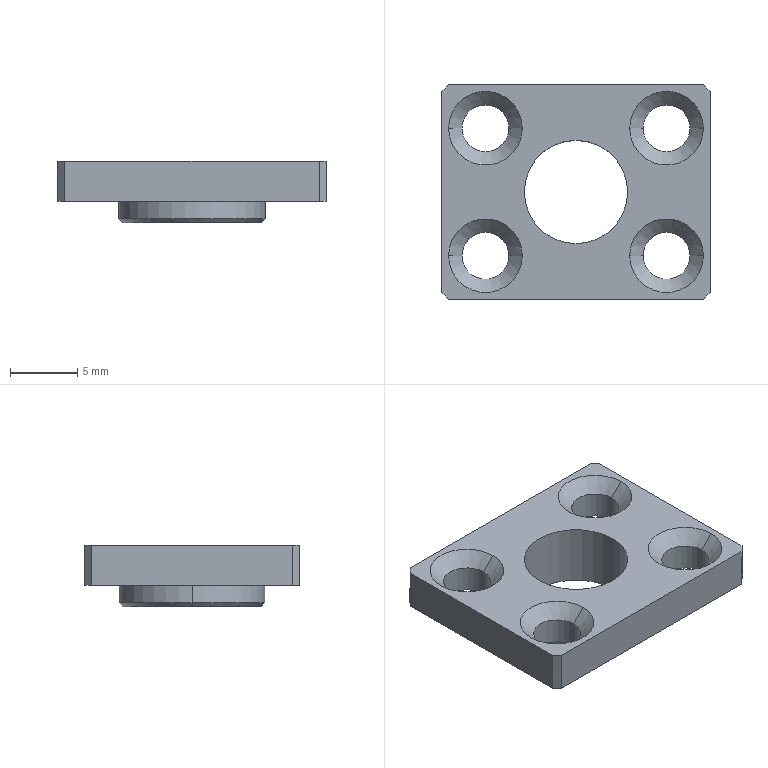Part | SolidWorks | features Chamfer 3, Extrusion 1, ICE 1 | 1 solid | 33 faces | box 20 x 16 x 4.6 mm | volume 750.45 mm3 | cylinder 12 | plane 11 | cone 10 | commonest cylinder face diameters 3.5 x8 7.7 x2 10.9 x2
STEP:
#1=CARTESIAN_POINT('',(-8.5,4.75,3.6));
#2=VERTEX_POINT('',#1);
#3=CARTESIAN_POINT('',(-5.,4.75,3.6));
#4=VERTEX_POINT('',#3);
#5=CARTESIAN_POINT('',(-6.75,4.75,3.6));
#6=DIRECTION('',(0.,0.,1.));
#7=DIRECTION('',(1.,0.,0.));
#8=AXIS2_PLACEMENT_3D('',#5,#6,#7);
#9=CIRCLE('',#8,1.75);
#10=EDGE_CURVE('',#2,#4,#9,.T.);
#11=ORIENTED_EDGE('',*,*,#10,.F.);
#12=CARTESIAN_POINT('',(-9.5,4.75,4.6));
#13=VERTEX_POINT('',#12);
#14=CARTESIAN_POINT('',(-8.5,4.75,3.6));
#15=DIRECTION('',(-0.7071,0.,0.7071));
#16=VECTOR('',#15,1000.);
#17=LINE('',#14,#16);
#18=EDGE_CURVE('',#2,#13,#17,.T.);
#19=ORIENTED_EDGE('',*,*,#18,.T.);
#20=CARTESIAN_POINT('',(-4.,4.75,4.6));
#21=VERTEX_POINT('',#20);
#22=CARTESIAN_POINT('',(-6.75,4.75,4.6));
#23=DIRECTION('',(0.,0.,-1.));
#24=DIRECTION('',(1.,0.,0.));
#25=AXIS2_PLACEMENT_3D('',#22,#23,#24);
#26=CIRCLE('',#25,2.75);
#27=EDGE_CURVE('',#21,#13,#26,.T.);
#28=ORIENTED_EDGE('',*,*,#27,.F.);
#29=CARTESIAN_POINT('',(-5.,4.75,3.6));
#30=DIRECTION('',(0.7071,0.,0.7071));
#31=VECTOR('',#30,1000.);
#32=LINE('',#29,#31);
#33=EDGE_CURVE('',#4,#21,#32,.T.);
#34=ORIENTED_EDGE('',*,*,#33,.F.);
#35=EDGE_LOOP('',(#11,#19,#28,#34));
#36=FACE_OUTER_BOUND('',#35,.T.);
#37=CARTESIAN_POINT('',(-6.75,4.75,3.6));
#38=DIRECTION('',(0.,0.,1.));
#39=DIRECTION('',(1.,0.,0.));
#40=AXIS2_PLACEMENT_3D('',#37,#38,#39);
#41=CONICAL_SURFACE('',#40,1.75,0.7854);
#42=ADVANCED_FACE('',(#36),#41,.F.);
#43=CARTESIAN_POINT('',(5.,4.75,3.6));
#44=VERTEX_POINT('',#43);
#45=CARTESIAN_POINT('',(8.5,4.75,3.6));
#46=VERTEX_POINT('',#45);
#47=CARTESIAN_POINT('',(6.75,4.75,3.6));
#48=DIRECTION('',(0.,0.,1.));
#49=DIRECTION('',(1.,0.,0.));
#50=AXIS2_PLACEMENT_3D('',#47,#48,#49);
#51=CIRCLE('',#50,1.75);
#52=EDGE_CURVE('',#44,#46,#51,.T.);
#53=ORIENTED_EDGE('',*,*,#52,.F.);
#54=CARTESIAN_POINT('',(4.,4.75,4.6));
#55=VERTEX_POINT('',#54);
#56=CARTESIAN_POINT('',(5.,4.75,3.6));
#57=DIRECTION('',(-0.7071,0.,0.7071));
#58=VECTOR('',#57,1000.);
#59=LINE('',#56,#58);
#60=EDGE_CURVE('',#44,#55,#59,.T.);
#61=ORIENTED_EDGE('',*,*,#60,.T.);
#62=CARTESIAN_POINT('',(9.5,4.75,4.6));
#63=VERTEX_POINT('',#62);
#64=CARTESIAN_POINT('',(6.75,4.75,4.6));
#65=DIRECTION('',(0.,0.,-1.));
#66=DIRECTION('',(1.,0.,0.));
#67=AXIS2_PLACEMENT_3D('',#64,#65,#66);
#68=CIRCLE('',#67,2.75);
#69=EDGE_CURVE('',#63,#55,#68,.T.);
#70=ORIENTED_EDGE('',*,*,#69,.F.);
#71=CARTESIAN_POINT('',(8.5,4.75,3.6));
#72=DIRECTION('',(0.7071,0.,0.7071));
#73=VECTOR('',#72,1000.);
#74=LINE('',#71,#73);
#75=EDGE_CURVE('',#46,#63,#74,.T.);
#76=ORIENTED_EDGE('',*,*,#75,.F.);
#77=EDGE_LOOP('',(#53,#61,#70,#76));
#78=FACE_OUTER_BOUND('',#77,.T.);
#79=CARTESIAN_POINT('',(6.75,4.75,3.6));
#80=DIRECTION('',(0.,0.,1.));
#81=DIRECTION('',(1.,0.,0.));
#82=AXIS2_PLACEMENT_3D('',#79,#80,#81);
#83=CONICAL_SURFACE('',#82,1.75,0.7854);
#84=ADVANCED_FACE('',(#78),#83,.F.);
#85=CARTESIAN_POINT('',(-8.5,-4.75,3.6));
#86=VERTEX_POINT('',#85);
#87=CARTESIAN_POINT('',(-5.,-4.75,3.6));
#88=VERTEX_POINT('',#87);
#89=CARTESIAN_POINT('',(-6.75,-4.75,3.6));
#90=DIRECTION('',(0.,0.,1.));
#91=DIRECTION('',(1.,0.,0.));
#92=AXIS2_PLACEMENT_3D('',#89,#90,#91);
#93=CIRCLE('',#92,1.75);
#94=EDGE_CURVE('',#86,#88,#93,.T.);
#95=ORIENTED_EDGE('',*,*,#94,.F.);
#96=CARTESIAN_POINT('',(-9.5,-4.75,4.6));
#97=VERTEX_POINT('',#96);
#98=CARTESIAN_POINT('',(-8.5,-4.75,3.6));
#99=DIRECTION('',(-0.7071,0.,0.7071));
#100=VECTOR('',#99,1000.);
#101=LINE('',#98,#100);
#102=EDGE_CURVE('',#86,#97,#101,.T.);
#103=ORIENTED_EDGE('',*,*,#102,.T.);
#104=CARTESIAN_POINT('',(-4.,-4.75,4.6));
#105=VERTEX_POINT('',#104);
#106=CARTESIAN_POINT('',(-6.75,-4.75,4.6));
#107=DIRECTION('',(0.,0.,-1.));
#108=DIRECTION('',(1.,0.,0.));
#109=AXIS2_PLACEMENT_3D('',#106,#107,#108);
#110=CIRCLE('',#109,2.75);
#111=EDGE_CURVE('',#105,#97,#110,.T.);
#112=ORIENTED_EDGE('',*,*,#111,.F.);
#113=CARTESIAN_POINT('',(-5.,-4.75,3.6));
#114=DIRECTION('',(0.7071,0.,0.7071));
#115=VECTOR('',#114,1000.);
#116=LINE('',#113,#115);
#117=EDGE_CURVE('',#88,#105,#116,.T.);
#118=ORIENTED_EDGE('',*,*,#117,.F.);
#119=EDGE_LOOP('',(#95,#103,#112,#118));
#120=FACE_OUTER_BOUND('',#119,.T.);
#121=CARTESIAN_POINT('',(-6.75,-4.75,3.6));
#122=DIRECTION('',(0.,0.,1.));
#123=DIRECTION('',(1.,0.,0.));
#124=AXIS2_PLACEMENT_3D('',#121,#122,#123);
#125=CONICAL_SURFACE('',#124,1.75,0.7854);
#126=ADVANCED_FACE('',(#120),#125,.F.);
#127=CARTESIAN_POINT('',(5.,-4.75,3.6));
#128=VERTEX_POINT('',#127);
#129=CARTESIAN_POINT('',(8.5,-4.75,3.6));
#130=VERTEX_POINT('',#129);
#131=CARTESIAN_POINT('',(6.75,-4.75,3.6));
#132=DIRECTION('',(0.,0.,1.));
#133=DIRECTION('',(1.,0.,0.));
#134=AXIS2_PLACEMENT_3D('',#131,#132,#133);
#135=CIRCLE('',#134,1.75);
#136=EDGE_CURVE('',#128,#130,#135,.T.);
#137=ORIENTED_EDGE('',*,*,#136,.F.);
#138=CARTESIAN_POINT('',(4.,-4.75,4.6));
#139=VERTEX_POINT('',#138);
#140=CARTESIAN_POINT('',(5.,-4.75,3.6));
#141=DIRECTION('',(-0.7071,0.,0.7071));
#142=VECTOR('',#141,1000.);
#143=LINE('',#140,#142);
#144=EDGE_CURVE('',#128,#139,#143,.T.);
#145=ORIENTED_EDGE('',*,*,#144,.T.);
#146=CARTESIAN_POINT('',(9.5,-4.75,4.6));
#147=VERTEX_POINT('',#146);
#148=CARTESIAN_POINT('',(6.75,-4.75,4.6));
#149=DIRECTION('',(0.,0.,-1.));
#150=DIRECTION('',(1.,0.,0.));
#151=AXIS2_PLACEMENT_3D('',#148,#149,#150);
#152=CIRCLE('',#151,2.75);
#153=EDGE_CURVE('',#147,#139,#152,.T.);
#154=ORIENTED_EDGE('',*,*,#153,.F.);
#155=CARTESIAN_POINT('',(8.5,-4.75,3.6));
#156=DIRECTION('',(0.7071,0.,0.7071));
#157=VECTOR('',#156,1000.);
#158=LINE('',#155,#157);
#159=EDGE_CURVE('',#130,#147,#158,.T.);
#160=ORIENTED_EDGE('',*,*,#159,.F.);
#161=EDGE_LOOP('',(#137,#145,#154,#160));
#162=FACE_OUTER_BOUND('',#161,.T.);
#163=CARTESIAN_POINT('',(6.75,-4.75,3.6));
#164=DIRECTION('',(0.,0.,1.));
#165=DIRECTION('',(1.,0.,0.));
#166=AXIS2_PLACEMENT_3D('',#163,#164,#165);
#167=CONICAL_SURFACE('',#166,1.75,0.7854);
#168=ADVANCED_FACE('',(#162),#167,.F.);
#169=CARTESIAN_POINT('',(-5.15,0.,0.));
#170=VERTEX_POINT('',#169);
#171=CARTESIAN_POINT('',(5.15,0.,0.));
#172=VERTEX_POINT('',#171);
#173=CARTESIAN_POINT('',(0.,0.,0.));
#174=DIRECTION('',(0.,0.,-1.));
#175=DIRECTION('',(1.,0.,0.));
#176=AXIS2_PLACEMENT_3D('',#173,#174,#175);
#177=CIRCLE('',#176,5.15);
#178=EDGE_CURVE('',#170,#172,#177,.T.);
#179=ORIENTED_EDGE('',*,*,#178,.F.);
#180=CARTESIAN_POINT('',(-5.45,0.,0.3));
#181=VERTEX_POINT('',#180);
#182=CARTESIAN_POINT('',(-5.45,0.,0.3));
#183=DIRECTION('',(-0.7071,0.,0.7071));
#184=VECTOR('',#183,1000.);
#185=LINE('',#182,#184);
#186=EDGE_CURVE('',#170,#181,#185,.T.);
#187=ORIENTED_EDGE('',*,*,#186,.T.);
#188=CARTESIAN_POINT('',(5.45,0.,0.3));
#189=VERTEX_POINT('',#188);
#190=CARTESIAN_POINT('',(0.,0.,0.3));
#191=DIRECTION('',(0.,0.,1.));
#192=DIRECTION('',(1.,0.,0.));
#193=AXIS2_PLACEMENT_3D('',#190,#191,#192);
#194=CIRCLE('',#193,5.45);
#195=EDGE_CURVE('',#189,#181,#194,.T.);
#196=ORIENTED_EDGE('',*,*,#195,.F.);
#197=CARTESIAN_POINT('',(5.45,0.,0.3));
#198=DIRECTION('',(0.7071,0.,0.7071));
#199=VECTOR('',#198,1000.);
#200=LINE('',#197,#199);
#201=EDGE_CURVE('',#172,#189,#200,.T.);
#202=ORIENTED_EDGE('',*,*,#201,.F.);
#203=EDGE_LOOP('',(#179,#187,#196,#202));
#204=FACE_OUTER_BOUND('',#203,.T.);
#205=CARTESIAN_POINT('',(0.,0.,0.3));
#206=DIRECTION('',(0.,0.,1.));
#207=DIRECTION('',(1.,0.,0.));
#208=AXIS2_PLACEMENT_3D('',#205,#206,#207);
#209=CONICAL_SURFACE('',#208,5.45,0.7854);
#210=ADVANCED_FACE('',(#204),#209,.T.);
#211=ORIENTED_EDGE('',*,*,#52,.T.);
#212=CARTESIAN_POINT('',(8.5,4.75,1.6));
#213=VERTEX_POINT('',#212);
#214=CARTESIAN_POINT('',(8.5,4.75,4.6));
#215=DIRECTION('',(0.,0.,-1.));
#216=VECTOR('',#215,1000.);
#217=LINE('',#214,#216);
#218=EDGE_CURVE('',#46,#213,#217,.T.);
#219=ORIENTED_EDGE('',*,*,#218,.T.);
#220=CARTESIAN_POINT('',(5.,4.75,1.6));
#221=VERTEX_POINT('',#220);
#222=CARTESIAN_POINT('',(6.75,4.75,1.6));
#223=DIRECTION('',(0.,0.,1.));
#224=DIRECTION('',(1.,0.,0.));
#225=AXIS2_PLACEMENT_3D('',#222,#223,#224);
#226=CIRCLE('',#225,1.75);
#227=EDGE_CURVE('',#221,#213,#226,.T.);
#228=ORIENTED_EDGE('',*,*,#227,.F.);
#229=CARTESIAN_POINT('',(5.,4.75,4.6));
#230=DIRECTION('',(0.,0.,-1.));
#231=VECTOR('',#230,1000.);
#232=LINE('',#229,#231);
#233=EDGE_CURVE('',#44,#221,#232,.T.);
#234=ORIENTED_EDGE('',*,*,#233,.F.);
#235=EDGE_LOOP('',(#211,#219,#228,#234));
#236=FACE_OUTER_BOUND('',#235,.T.);
#237=CARTESIAN_POINT('',(6.75,4.75,4.6));
#238=DIRECTION('',(0.,0.,-1.));
#239=DIRECTION('',(-1.,0.,0.));
#240=AXIS2_PLACEMENT_3D('',#237,#238,#239);
#241=CYLINDRICAL_SURFACE('',#240,1.75);
#242=ADVANCED_FACE('',(#236),#241,.F.);
#243=ORIENTED_EDGE('',*,*,#136,.T.);
#244=CARTESIAN_POINT('',(8.5,-4.75,1.6));
#245=VERTEX_POINT('',#244);
#246=CARTESIAN_POINT('',(8.5,-4.75,4.6));
#247=DIRECTION('',(0.,0.,-1.));
#248=VECTOR('',#247,1000.);
#249=LINE('',#246,#248);
#250=EDGE_CURVE('',#130,#245,#249,.T.);
#251=ORIENTED_EDGE('',*,*,#250,.T.);
#252=CARTESIAN_POINT('',(5.,-4.75,1.6));
#253=VERTEX_POINT('',#252);
#254=CARTESIAN_POINT('',(6.75,-4.75,1.6));
#255=DIRECTION('',(0.,0.,1.));
#256=DIRECTION('',(1.,0.,0.));
#257=AXIS2_PLACEMENT_3D('',#254,#255,#256);
#258=CIRCLE('',#257,1.75);
#259=EDGE_CURVE('',#253,#245,#258,.T.);
#260=ORIENTED_EDGE('',*,*,#259,.F.);
#261=CARTESIAN_POINT('',(5.,-4.75,4.6));
#262=DIRECTION('',(0.,0.,-1.));
#263=VECTOR('',#262,1000.);
#264=LINE('',#261,#263);
#265=EDGE_CURVE('',#128,#253,#264,.T.);
#266=ORIENTED_EDGE('',*,*,#265,.F.);
#267=EDGE_LOOP('',(#243,#251,#260,#266));
#268=FACE_OUTER_BOUND('',#267,.T.);
#269=CARTESIAN_POINT('',(6.75,-4.75,4.6));
#270=DIRECTION('',(0.,0.,-1.));
#271=DIRECTION('',(-1.,0.,0.));
#272=AXIS2_PLACEMENT_3D('',#269,#270,#271);
#273=CYLINDRICAL_SURFACE('',#272,1.75);
#274=ADVANCED_FACE('',(#268),#273,.F.);
#275=ORIENTED_EDGE('',*,*,#94,.T.);
#276=CARTESIAN_POINT('',(-5.,-4.75,1.6));
#277=VERTEX_POINT('',#276);
#278=CARTESIAN_POINT('',(-5.,-4.75,4.6));
#279=DIRECTION('',(0.,0.,-1.));
#280=VECTOR('',#279,1000.);
#281=LINE('',#278,#280);
#282=EDGE_CURVE('',#88,#277,#281,.T.);
#283=ORIENTED_EDGE('',*,*,#282,.T.);
#284=CARTESIAN_POINT('',(-8.5,-4.75,1.6));
#285=VERTEX_POINT('',#284);
#286=CARTESIAN_POINT('',(-6.75,-4.75,1.6));
#287=DIRECTION('',(0.,0.,1.));
#288=DIRECTION('',(1.,0.,0.));
#289=AXIS2_PLACEMENT_3D('',#286,#287,#288);
#290=CIRCLE('',#289,1.75);
#291=EDGE_CURVE('',#285,#277,#290,.T.);
#292=ORIENTED_EDGE('',*,*,#291,.F.);
#293=CARTESIAN_POINT('',(-8.5,-4.75,4.6));
#294=DIRECTION('',(0.,0.,-1.));
#295=VECTOR('',#294,1000.);
#296=LINE('',#293,#295);
#297=EDGE_CURVE('',#86,#285,#296,.T.);
#298=ORIENTED_EDGE('',*,*,#297,.F.);
#299=EDGE_LOOP('',(#275,#283,#292,#298));
#300=FACE_OUTER_BOUND('',#299,.T.);
#301=CARTESIAN_POINT('',(-6.75,-4.75,4.6));
#302=DIRECTION('',(0.,0.,-1.));
#303=DIRECTION('',(-1.,0.,0.));
#304=AXIS2_PLACEMENT_3D('',#301,#302,#303);
#305=CYLINDRICAL_SURFACE('',#304,1.75);
#306=ADVANCED_FACE('',(#300),#305,.F.);
#307=ORIENTED_EDGE('',*,*,#10,.T.);
#308=CARTESIAN_POINT('',(-5.,4.75,1.6));
#309=VERTEX_POINT('',#308);
#310=CARTESIAN_POINT('',(-5.,4.75,4.6));
#311=DIRECTION('',(0.,0.,-1.));
#312=VECTOR('',#311,1000.);
#313=LINE('',#310,#312);
#314=EDGE_CURVE('',#4,#309,#313,.T.);
#315=ORIENTED_EDGE('',*,*,#314,.T.);
#316=CARTESIAN_POINT('',(-8.5,4.75,1.6));
#317=VERTEX_POINT('',#316);
#318=CARTESIAN_POINT('',(-6.75,4.75,1.6));
#319=DIRECTION('',(0.,0.,1.));
#320=DIRECTION('',(1.,0.,0.));
#321=AXIS2_PLACEMENT_3D('',#318,#319,#320);
#322=CIRCLE('',#321,1.75);
#323=EDGE_CURVE('',#317,#309,#322,.T.);
#324=ORIENTED_EDGE('',*,*,#323,.F.);
#325=CARTESIAN_POINT('',(-8.5,4.75,4.6));
#326=DIRECTION('',(0.,0.,-1.));
#327=VECTOR('',#326,1000.);
#328=LINE('',#325,#327);
#329=EDGE_CURVE('',#2,#317,#328,.T.);
#330=ORIENTED_EDGE('',*,*,#329,.F.);
#331=EDGE_LOOP('',(#307,#315,#324,#330));
#332=FACE_OUTER_BOUND('',#331,.T.);
#333=CARTESIAN_POINT('',(-6.75,4.75,4.6));
#334=DIRECTION('',(0.,0.,-1.));
#335=DIRECTION('',(-1.,0.,0.));
#336=AXIS2_PLACEMENT_3D('',#333,#334,#335);
#337=CYLINDRICAL_SURFACE('',#336,1.75);
#338=ADVANCED_FACE('',(#332),#337,.F.);
#339=CARTESIAN_POINT('',(-3.85,0.,4.6));
#340=VERTEX_POINT('',#339);
#341=CARTESIAN_POINT('',(3.85,0.,4.6));
#342=VERTEX_POINT('',#341);
#343=CARTESIAN_POINT('',(0.,0.,4.6));
#344=DIRECTION('',(0.,0.,1.));
#345=DIRECTION('',(1.,0.,0.));
#346=AXIS2_PLACEMENT_3D('',#343,#344,#345);
#347=CIRCLE('',#346,3.85);
#348=EDGE_CURVE('',#340,#342,#347,.T.);
#349=ORIENTED_EDGE('',*,*,#348,.T.);
#350=CARTESIAN_POINT('',(3.85,0.,0.));
#351=VERTEX_POINT('',#350);
#352=CARTESIAN_POINT('',(3.85,0.,1.6));
#353=DIRECTION('',(0.,0.,-1.));
#354=VECTOR('',#353,1000.);
#355=LINE('',#352,#354);
#356=EDGE_CURVE('',#342,#351,#355,.T.);
#357=ORIENTED_EDGE('',*,*,#356,.T.);
#358=CARTESIAN_POINT('',(-3.85,0.,0.));
#359=VERTEX_POINT('',#358);
#360=CARTESIAN_POINT('',(0.,0.,0.));
#361=DIRECTION('',(0.,0.,1.));
#362=DIRECTION('',(1.,0.,0.));
#363=AXIS2_PLACEMENT_3D('',#360,#361,#362);
#364=CIRCLE('',#363,3.85);
#365=EDGE_CURVE('',#359,#351,#364,.T.);
#366=ORIENTED_EDGE('',*,*,#365,.F.);
#367=CARTESIAN_POINT('',(-3.85,0.,1.6));
#368=DIRECTION('',(0.,0.,-1.));
#369=VECTOR('',#368,1000.);
#370=LINE('',#367,#369);
#371=EDGE_CURVE('',#340,#359,#370,.T.);
#372=ORIENTED_EDGE('',*,*,#371,.F.);
#373=EDGE_LOOP('',(#349,#357,#366,#372));
#374=FACE_OUTER_BOUND('',#373,.T.);
#375=CARTESIAN_POINT('',(0.,0.,1.6));
#376=DIRECTION('',(0.,0.,-1.));
#377=DIRECTION('',(-1.,0.,0.));
#378=AXIS2_PLACEMENT_3D('',#375,#376,#377);
#379=CYLINDRICAL_SURFACE('',#378,3.85);
#380=ADVANCED_FACE('',(#374),#379,.F.);
#381=CARTESIAN_POINT('',(5.45,0.,1.6));
#382=VERTEX_POINT('',#381);
#383=CARTESIAN_POINT('',(-5.45,0.,1.6));
#384=VERTEX_POINT('',#383);
#385=CARTESIAN_POINT('',(0.,0.,1.6));
#386=DIRECTION('',(0.,0.,1.));
#387=DIRECTION('',(1.,0.,0.));
#388=AXIS2_PLACEMENT_3D('',#385,#386,#387);
#389=CIRCLE('',#388,5.45);
#390=EDGE_CURVE('',#382,#384,#389,.T.);
#391=ORIENTED_EDGE('',*,*,#390,.F.);
#392=CARTESIAN_POINT('',(5.45,0.,1.6));
#393=DIRECTION('',(0.,0.,-1.));
#394=VECTOR('',#393,1000.);
#395=LINE('',#392,#394);
#396=EDGE_CURVE('',#382,#189,#395,.T.);
#397=ORIENTED_EDGE('',*,*,#396,.T.);
#398=ORIENTED_EDGE('',*,*,#195,.T.);
#399=CARTESIAN_POINT('',(-5.45,0.,1.6));
#400=DIRECTION('',(0.,0.,-1.));
#401=VECTOR('',#400,1000.);
#402=LINE('',#399,#401);
#403=EDGE_CURVE('',#384,#181,#402,.T.);
#404=ORIENTED_EDGE('',*,*,#403,.F.);
#405=EDGE_LOOP('',(#391,#397,#398,#404));
#406=FACE_OUTER_BOUND('',#405,.T.);
#407=CARTESIAN_POINT('',(0.,0.,1.6));
#408=DIRECTION('',(0.,0.,-1.));
#409=DIRECTION('',(-1.,0.,0.));
#410=AXIS2_PLACEMENT_3D('',#407,#408,#409);
#411=CYLINDRICAL_SURFACE('',#410,5.45);
#412=ADVANCED_FACE('',(#406),#411,.T.);
#413=CARTESIAN_POINT('',(0.,0.,0.));
#414=DIRECTION('',(0.,0.,-1.));
#415=DIRECTION('',(1.,0.,0.));
#416=AXIS2_PLACEMENT_3D('',#413,#414,#415);
#417=CIRCLE('',#416,5.15);
#418=EDGE_CURVE('',#172,#170,#417,.T.);
#419=ORIENTED_EDGE('',*,*,#418,.T.);
#420=ORIENTED_EDGE('',*,*,#178,.T.);
#421=EDGE_LOOP('',(#419,#420));
#422=FACE_OUTER_BOUND('',#421,.T.);
#423=ORIENTED_EDGE('',*,*,#365,.T.);
#424=CARTESIAN_POINT('',(0.,0.,0.));
#425=DIRECTION('',(0.,0.,1.));
#426=DIRECTION('',(1.,0.,0.));
#427=AXIS2_PLACEMENT_3D('',#424,#425,#426);
#428=CIRCLE('',#427,3.85);
#429=EDGE_CURVE('',#351,#359,#428,.T.);
#430=ORIENTED_EDGE('',*,*,#429,.T.);
#431=EDGE_LOOP('',(#423,#430));
#432=FACE_BOUND('',#431,.T.);
#433=CARTESIAN_POINT('',(0.,0.,0.));
#434=DIRECTION('',(0.,0.,1.));
#435=DIRECTION('',(1.,0.,0.));
#436=AXIS2_PLACEMENT_3D('',#433,#434,#435);
#437=PLANE('',#436);
#438=ADVANCED_FACE('',(#422,#432),#437,.F.);
#439=ORIENTED_EDGE('',*,*,#396,.F.);
#440=CARTESIAN_POINT('',(0.,0.,1.6));
#441=DIRECTION('',(0.,0.,1.));
#442=DIRECTION('',(1.,0.,0.));
#443=AXIS2_PLACEMENT_3D('',#440,#441,#442);
#444=CIRCLE('',#443,5.45);
#445=EDGE_CURVE('',#384,#382,#444,.T.);
#446=ORIENTED_EDGE('',*,*,#445,.F.);
#447=ORIENTED_EDGE('',*,*,#403,.T.);
#448=CARTESIAN_POINT('',(0.,0.,0.3));
#449=DIRECTION('',(0.,0.,1.));
#450=DIRECTION('',(1.,0.,0.));
#451=AXIS2_PLACEMENT_3D('',#448,#449,#450);
#452=CIRCLE('',#451,5.45);
#453=EDGE_CURVE('',#181,#189,#452,.T.);
#454=ORIENTED_EDGE('',*,*,#453,.T.);
#455=EDGE_LOOP('',(#439,#446,#447,#454));
#456=FACE_OUTER_BOUND('',#455,.T.);
#457=CARTESIAN_POINT('',(0.,0.,1.6));
#458=DIRECTION('',(0.,0.,-1.));
#459=DIRECTION('',(-1.,0.,0.));
#460=AXIS2_PLACEMENT_3D('',#457,#458,#459);
#461=CYLINDRICAL_SURFACE('',#460,5.45);
#462=ADVANCED_FACE('',(#456),#461,.T.);
#463=ORIENTED_EDGE('',*,*,#356,.F.);
#464=CARTESIAN_POINT('',(0.,0.,4.6));
#465=DIRECTION('',(0.,0.,1.));
#466=DIRECTION('',(1.,0.,0.));
#467=AXIS2_PLACEMENT_3D('',#464,#465,#466);
#468=CIRCLE('',#467,3.85);
#469=EDGE_CURVE('',#342,#340,#468,.T.);
#470=ORIENTED_EDGE('',*,*,#469,.T.);
#471=ORIENTED_EDGE('',*,*,#371,.T.);
#472=ORIENTED_EDGE('',*,*,#429,.F.);
#473=EDGE_LOOP('',(#463,#470,#471,#472));
#474=FACE_OUTER_BOUND('',#473,.T.);
#475=CARTESIAN_POINT('',(0.,0.,1.6));
#476=DIRECTION('',(0.,0.,-1.));
#477=DIRECTION('',(-1.,0.,0.));
#478=AXIS2_PLACEMENT_3D('',#475,#476,#477);
#479=CYLINDRICAL_SURFACE('',#478,3.85);
#480=ADVANCED_FACE('',(#474),#479,.F.);
#481=ORIENTED_EDGE('',*,*,#153,.T.);
#482=CARTESIAN_POINT('',(6.75,-4.75,4.6));
#483=DIRECTION('',(0.,0.,-1.));
#484=DIRECTION('',(1.,0.,0.));
#485=AXIS2_PLACEMENT_3D('',#482,#483,#484);
#486=CIRCLE('',#485,2.75);
#487=EDGE_CURVE('',#139,#147,#486,.T.);
#488=ORIENTED_EDGE('',*,*,#487,.T.);
#489=EDGE_LOOP('',(#481,#488));
#490=FACE_BOUND('',#489,.T.);
#491=ORIENTED_EDGE('',*,*,#111,.T.);
#492=CARTESIAN_POINT('',(-6.75,-4.75,4.6));
#493=DIRECTION('',(0.,0.,-1.));
#494=DIRECTION('',(1.,0.,0.));
#495=AXIS2_PLACEMENT_3D('',#492,#493,#494);
#496=CIRCLE('',#495,2.75);
#497=EDGE_CURVE('',#97,#105,#496,.T.);
#498=ORIENTED_EDGE('',*,*,#497,.T.);
#499=EDGE_LOOP('',(#491,#498));
#500=FACE_BOUND('',#499,.T.);
#501=ORIENTED_EDGE('',*,*,#69,.T.);
#502=CARTESIAN_POINT('',(6.75,4.75,4.6));
#503=DIRECTION('',(0.,0.,-1.));
#504=DIRECTION('',(1.,0.,0.));
#505=AXIS2_PLACEMENT_3D('',#502,#503,#504);
#506=CIRCLE('',#505,2.75);
#507=EDGE_CURVE('',#55,#63,#506,.T.);
#508=ORIENTED_EDGE('',*,*,#507,.T.);
#509=EDGE_LOOP('',(#501,#508));
#510=FACE_BOUND('',#509,.T.);
#511=ORIENTED_EDGE('',*,*,#27,.T.);
#512=CARTESIAN_POINT('',(-6.75,4.75,4.6));
#513=DIRECTION('',(0.,0.,-1.));
#514=DIRECTION('',(1.,0.,0.));
#515=AXIS2_PLACEMENT_3D('',#512,#513,#514);
#516=CIRCLE('',#515,2.75);
#517=EDGE_CURVE('',#13,#21,#516,.T.);
#518=ORIENTED_EDGE('',*,*,#517,.T.);
#519=EDGE_LOOP('',(#511,#518));
#520=FACE_BOUND('',#519,.T.);
#521=ORIENTED_EDGE('',*,*,#348,.F.);
#522=ORIENTED_EDGE('',*,*,#469,.F.);
#523=EDGE_LOOP('',(#521,#522));
#524=FACE_BOUND('',#523,.T.);
#525=CARTESIAN_POINT('',(-10.,7.5,4.6));
#526=VERTEX_POINT('',#525);
#527=CARTESIAN_POINT('',(-10.,-7.5,4.6));
#528=VERTEX_POINT('',#527);
#529=CARTESIAN_POINT('',(-10.,8.,4.6));
#530=DIRECTION('',(0.,-1.,0.));
#531=VECTOR('',#530,1000.);
#532=LINE('',#529,#531);
#533=EDGE_CURVE('',#526,#528,#532,.T.);
#534=ORIENTED_EDGE('',*,*,#533,.T.);
#535=CARTESIAN_POINT('',(-9.5,-8.,4.6));
#536=VERTEX_POINT('',#535);
#537=CARTESIAN_POINT('',(-8.75,-8.75,4.6));
#538=DIRECTION('',(0.7071,-0.7071,0.));
#539=VECTOR('',#538,1000.);
#540=LINE('',#537,#539);
#541=EDGE_CURVE('',#528,#536,#540,.T.);
#542=ORIENTED_EDGE('',*,*,#541,.T.);
#543=CARTESIAN_POINT('',(9.5,-8.,4.6));
#544=VERTEX_POINT('',#543);
#545=CARTESIAN_POINT('',(-10.,-8.,4.6));
#546=DIRECTION('',(1.,0.,0.));
#547=VECTOR('',#546,1000.);
#548=LINE('',#545,#547);
#549=EDGE_CURVE('',#536,#544,#548,.T.);
#550=ORIENTED_EDGE('',*,*,#549,.T.);
#551=CARTESIAN_POINT('',(10.,-7.5,4.6));
#552=VERTEX_POINT('',#551);
#553=CARTESIAN_POINT('',(8.75,-8.75,4.6));
#554=DIRECTION('',(0.7071,0.7071,0.));
#555=VECTOR('',#554,1000.);
#556=LINE('',#553,#555);
#557=EDGE_CURVE('',#544,#552,#556,.T.);
#558=ORIENTED_EDGE('',*,*,#557,.T.);
#559=CARTESIAN_POINT('',(10.,7.5,4.6));
#560=VERTEX_POINT('',#559);
#561=CARTESIAN_POINT('',(10.,8.,4.6));
#562=DIRECTION('',(0.,1.,0.));
#563=VECTOR('',#562,1000.);
#564=LINE('',#561,#563);
#565=EDGE_CURVE('',#552,#560,#564,.T.);
#566=ORIENTED_EDGE('',*,*,#565,.T.);
#567=CARTESIAN_POINT('',(9.5,8.,4.6));
#568=VERTEX_POINT('',#567);
#569=CARTESIAN_POINT('',(8.75,8.75,4.6));
#570=DIRECTION('',(-0.7071,0.7071,0.));
#571=VECTOR('',#570,1000.);
#572=LINE('',#569,#571);
#573=EDGE_CURVE('',#560,#568,#572,.T.);
#574=ORIENTED_EDGE('',*,*,#573,.T.);
#575=CARTESIAN_POINT('',(-9.5,8.,4.6));
#576=VERTEX_POINT('',#575);
#577=CARTESIAN_POINT('',(-10.,8.,4.6));
#578=DIRECTION('',(-1.,0.,0.));
#579=VECTOR('',#578,1000.);
#580=LINE('',#577,#579);
#581=EDGE_CURVE('',#568,#576,#580,.T.);
#582=ORIENTED_EDGE('',*,*,#581,.T.);
#583=CARTESIAN_POINT('',(-8.75,8.75,4.6));
#584=DIRECTION('',(-0.7071,-0.7071,0.));
#585=VECTOR('',#584,1000.);
#586=LINE('',#583,#585);
#587=EDGE_CURVE('',#576,#526,#586,.T.);
#588=ORIENTED_EDGE('',*,*,#587,.T.);
#589=EDGE_LOOP('',(#534,#542,#550,#558,#566,#574,#582,#588));
#590=FACE_OUTER_BOUND('',#589,.T.);
#591=CARTESIAN_POINT('',(0.,0.,4.6));
#592=DIRECTION('',(0.,0.,1.));
#593=DIRECTION('',(1.,0.,0.));
#594=AXIS2_PLACEMENT_3D('',#591,#592,#593);
#595=PLANE('',#594);
#596=ADVANCED_FACE('',(#490,#500,#510,#520,#524,#590),#595,.T.);
#597=ORIENTED_EDGE('',*,*,#445,.T.);
#598=ORIENTED_EDGE('',*,*,#390,.T.);
#599=EDGE_LOOP('',(#597,#598));
#600=FACE_BOUND('',#599,.T.);
#601=CARTESIAN_POINT('',(-9.5,-8.,1.6));
#602=VERTEX_POINT('',#601);
#603=CARTESIAN_POINT('',(9.5,-8.,1.6));
#604=VERTEX_POINT('',#603);
#605=CARTESIAN_POINT('',(-10.,-8.,1.6));
#606=DIRECTION('',(1.,0.,0.));
#607=VECTOR('',#606,1000.);
#608=LINE('',#605,#607);
#609=EDGE_CURVE('',#602,#604,#608,.T.);
#610=ORIENTED_EDGE('',*,*,#609,.F.);
#611=CARTESIAN_POINT('',(-10.,-7.5,1.6));
#612=VERTEX_POINT('',#611);
#613=CARTESIAN_POINT('',(-9.5,-8.,1.6));
#614=DIRECTION('',(-0.7071,0.7071,0.));
#615=VECTOR('',#614,1000.);
#616=LINE('',#613,#615);
#617=EDGE_CURVE('',#602,#612,#616,.T.);
#618=ORIENTED_EDGE('',*,*,#617,.T.);
#619=CARTESIAN_POINT('',(-10.,7.5,1.6));
#620=VERTEX_POINT('',#619);
#621=CARTESIAN_POINT('',(-10.,8.,1.6));
#622=DIRECTION('',(0.,-1.,0.));
#623=VECTOR('',#622,1000.);
#624=LINE('',#621,#623);
#625=EDGE_CURVE('',#620,#612,#624,.T.);
#626=ORIENTED_EDGE('',*,*,#625,.F.);
#627=CARTESIAN_POINT('',(-9.5,8.,1.6));
#628=VERTEX_POINT('',#627);
#629=CARTESIAN_POINT('',(-10.,7.5,1.6));
#630=DIRECTION('',(0.7071,0.7071,0.));
#631=VECTOR('',#630,1000.);
#632=LINE('',#629,#631);
#633=EDGE_CURVE('',#620,#628,#632,.T.);
#634=ORIENTED_EDGE('',*,*,#633,.T.);
#635=CARTESIAN_POINT('',(9.5,8.,1.6));
#636=VERTEX_POINT('',#635);
#637=CARTESIAN_POINT('',(-10.,8.,1.6));
#638=DIRECTION('',(-1.,0.,0.));
#639=VECTOR('',#638,1000.);
#640=LINE('',#637,#639);
#641=EDGE_CURVE('',#636,#628,#640,.T.);
#642=ORIENTED_EDGE('',*,*,#641,.F.);
#643=CARTESIAN_POINT('',(10.,7.5,1.6));
#644=VERTEX_POINT('',#643);
#645=CARTESIAN_POINT('',(9.5,8.,1.6));
#646=DIRECTION('',(0.7071,-0.7071,0.));
#647=VECTOR('',#646,1000.);
#648=LINE('',#645,#647);
#649=EDGE_CURVE('',#636,#644,#648,.T.);
#650=ORIENTED_EDGE('',*,*,#649,.T.);
#651=CARTESIAN_POINT('',(10.,-7.5,1.6));
#652=VERTEX_POINT('',#651);
#653=CARTESIAN_POINT('',(10.,8.,1.6));
#654=DIRECTION('',(0.,1.,0.));
#655=VECTOR('',#654,1000.);
#656=LINE('',#653,#655);
#657=EDGE_CURVE('',#652,#644,#656,.T.);
#658=ORIENTED_EDGE('',*,*,#657,.F.);
#659=CARTESIAN_POINT('',(10.,-7.5,1.6));
#660=DIRECTION('',(-0.7071,-0.7071,0.));
#661=VECTOR('',#660,1000.);
#662=LINE('',#659,#661);
#663=EDGE_CURVE('',#652,#604,#662,.T.);
#664=ORIENTED_EDGE('',*,*,#663,.T.);
#665=EDGE_LOOP('',(#610,#618,#626,#634,#642,#650,#658,#664));
#666=FACE_OUTER_BOUND('',#665,.T.);
#667=ORIENTED_EDGE('',*,*,#323,.T.);
#668=CARTESIAN_POINT('',(-6.75,4.75,1.6));
#669=DIRECTION('',(0.,0.,1.));
#670=DIRECTION('',(1.,0.,0.));
#671=AXIS2_PLACEMENT_3D('',#668,#669,#670);
#672=CIRCLE('',#671,1.75);
#673=EDGE_CURVE('',#309,#317,#672,.T.);
#674=ORIENTED_EDGE('',*,*,#673,.T.);
#675=EDGE_LOOP('',(#667,#674));
#676=FACE_BOUND('',#675,.T.);
#677=ORIENTED_EDGE('',*,*,#291,.T.);
#678=CARTESIAN_POINT('',(-6.75,-4.75,1.6));
#679=DIRECTION('',(0.,0.,1.));
#680=DIRECTION('',(1.,0.,0.));
#681=AXIS2_PLACEMENT_3D('',#678,#679,#680);
#682=CIRCLE('',#681,1.75);
#683=EDGE_CURVE('',#277,#285,#682,.T.);
#684=ORIENTED_EDGE('',*,*,#683,.T.);
#685=EDGE_LOOP('',(#677,#684));
#686=FACE_BOUND('',#685,.T.);
#687=ORIENTED_EDGE('',*,*,#259,.T.);
#688=CARTESIAN_POINT('',(6.75,-4.75,1.6));
#689=DIRECTION('',(0.,0.,1.));
#690=DIRECTION('',(1.,0.,0.));
#691=AXIS2_PLACEMENT_3D('',#688,#689,#690);
#692=CIRCLE('',#691,1.75);
#693=EDGE_CURVE('',#245,#253,#692,.T.);
#694=ORIENTED_EDGE('',*,*,#693,.T.);
#695=EDGE_LOOP('',(#687,#694));
#696=FACE_BOUND('',#695,.T.);
#697=ORIENTED_EDGE('',*,*,#227,.T.);
#698=CARTESIAN_POINT('',(6.75,4.75,1.6));
#699=DIRECTION('',(0.,0.,1.));
#700=DIRECTION('',(1.,0.,0.));
#701=AXIS2_PLACEMENT_3D('',#698,#699,#700);
#702=CIRCLE('',#701,1.75);
#703=EDGE_CURVE('',#213,#221,#702,.T.);
#704=ORIENTED_EDGE('',*,*,#703,.T.);
#705=EDGE_LOOP('',(#697,#704));
#706=FACE_BOUND('',#705,.T.);
#707=CARTESIAN_POINT('',(0.,0.,1.6));
#708=DIRECTION('',(0.,0.,1.));
#709=DIRECTION('',(1.,0.,0.));
#710=AXIS2_PLACEMENT_3D('',#707,#708,#709);
#711=PLANE('',#710);
#712=ADVANCED_FACE('',(#600,#666,#676,#686,#696,#706),#711,.F.);
#713=ORIENTED_EDGE('',*,*,#565,.F.);
#714=CARTESIAN_POINT('',(10.,-7.5,4.6));
#715=DIRECTION('',(0.,0.,-1.));
#716=VECTOR('',#715,1000.);
#717=LINE('',#714,#716);
#718=EDGE_CURVE('',#552,#652,#717,.T.);
#719=ORIENTED_EDGE('',*,*,#718,.T.);
#720=ORIENTED_EDGE('',*,*,#657,.T.);
#721=CARTESIAN_POINT('',(10.,7.5,4.6));
#722=DIRECTION('',(0.,0.,1.));
#723=VECTOR('',#722,1000.);
#724=LINE('',#721,#723);
#725=EDGE_CURVE('',#644,#560,#724,.T.);
#726=ORIENTED_EDGE('',*,*,#725,.T.);
#727=EDGE_LOOP('',(#713,#719,#720,#726));
#728=FACE_OUTER_BOUND('',#727,.T.);
#729=CARTESIAN_POINT('',(10.,8.,4.6));
#730=DIRECTION('',(-1.,0.,0.));
#731=DIRECTION('',(0.,-1.,0.));
#732=AXIS2_PLACEMENT_3D('',#729,#730,#731);
#733=PLANE('',#732);
#734=ADVANCED_FACE('',(#728),#733,.F.);
#735=ORIENTED_EDGE('',*,*,#581,.F.);
#736=CARTESIAN_POINT('',(9.5,8.,4.6));
#737=DIRECTION('',(0.,0.,-1.));
#738=VECTOR('',#737,1000.);
#739=LINE('',#736,#738);
#740=EDGE_CURVE('',#568,#636,#739,.T.);
#741=ORIENTED_EDGE('',*,*,#740,.T.);
#742=ORIENTED_EDGE('',*,*,#641,.T.);
#743=CARTESIAN_POINT('',(-9.5,8.,4.6));
#744=DIRECTION('',(0.,0.,1.));
#745=VECTOR('',#744,1000.);
#746=LINE('',#743,#745);
#747=EDGE_CURVE('',#628,#576,#746,.T.);
#748=ORIENTED_EDGE('',*,*,#747,.T.);
#749=EDGE_LOOP('',(#735,#741,#742,#748));
#750=FACE_OUTER_BOUND('',#749,.T.);
#751=CARTESIAN_POINT('',(-10.,8.,4.6));
#752=DIRECTION('',(0.,-1.,0.));
#753=DIRECTION('',(0.,0.,-1.));
#754=AXIS2_PLACEMENT_3D('',#751,#752,#753);
#755=PLANE('',#754);
#756=ADVANCED_FACE('',(#750),#755,.F.);
#757=ORIENTED_EDGE('',*,*,#625,.T.);
#758=CARTESIAN_POINT('',(-10.,-7.5,4.6));
#759=DIRECTION('',(0.,0.,1.));
#760=VECTOR('',#759,1000.);
#761=LINE('',#758,#760);
#762=EDGE_CURVE('',#612,#528,#761,.T.);
#763=ORIENTED_EDGE('',*,*,#762,.T.);
#764=ORIENTED_EDGE('',*,*,#533,.F.);
#765=CARTESIAN_POINT('',(-10.,7.5,4.6));
#766=DIRECTION('',(0.,0.,-1.));
#767=VECTOR('',#766,1000.);
#768=LINE('',#765,#767);
#769=EDGE_CURVE('',#526,#620,#768,.T.);
#770=ORIENTED_EDGE('',*,*,#769,.T.);
#771=EDGE_LOOP('',(#757,#763,#764,#770));
#772=FACE_OUTER_BOUND('',#771,.T.);
#773=CARTESIAN_POINT('',(-10.,8.,4.6));
#774=DIRECTION('',(1.,0.,0.));
#775=DIRECTION('',(0.,1.,0.));
#776=AXIS2_PLACEMENT_3D('',#773,#774,#775);
#777=PLANE('',#776);
#778=ADVANCED_FACE('',(#772),#777,.F.);
#779=ORIENTED_EDGE('',*,*,#549,.F.);
#780=CARTESIAN_POINT('',(-9.5,-8.,4.6));
#781=DIRECTION('',(0.,0.,-1.));
#782=VECTOR('',#781,1000.);
#783=LINE('',#780,#782);
#784=EDGE_CURVE('',#536,#602,#783,.T.);
#785=ORIENTED_EDGE('',*,*,#784,.T.);
#786=ORIENTED_EDGE('',*,*,#609,.T.);
#787=CARTESIAN_POINT('',(9.5,-8.,4.6));
#788=DIRECTION('',(0.,0.,1.));
#789=VECTOR('',#788,1000.);
#790=LINE('',#787,#789);
#791=EDGE_CURVE('',#604,#544,#790,.T.);
#792=ORIENTED_EDGE('',*,*,#791,.T.);
#793=EDGE_LOOP('',(#779,#785,#786,#792));
#794=FACE_OUTER_BOUND('',#793,.T.);
#795=CARTESIAN_POINT('',(-10.,-8.,4.6));
#796=DIRECTION('',(0.,1.,0.));
#797=DIRECTION('',(0.,0.,1.));
#798=AXIS2_PLACEMENT_3D('',#795,#796,#797);
#799=PLANE('',#798);
#800=ADVANCED_FACE('',(#794),#799,.F.);
#801=ORIENTED_EDGE('',*,*,#314,.F.);
#802=CARTESIAN_POINT('',(-6.75,4.75,3.6));
#803=DIRECTION('',(0.,0.,1.));
#804=DIRECTION('',(1.,0.,0.));
#805=AXIS2_PLACEMENT_3D('',#802,#803,#804);
#806=CIRCLE('',#805,1.75);
#807=EDGE_CURVE('',#4,#2,#806,.T.);
#808=ORIENTED_EDGE('',*,*,#807,.T.);
#809=ORIENTED_EDGE('',*,*,#329,.T.);
#810=ORIENTED_EDGE('',*,*,#673,.F.);
#811=EDGE_LOOP('',(#801,#808,#809,#810));
#812=FACE_OUTER_BOUND('',#811,.T.);
#813=CARTESIAN_POINT('',(-6.75,4.75,4.6));
#814=DIRECTION('',(0.,0.,-1.));
#815=DIRECTION('',(-1.,0.,0.));
#816=AXIS2_PLACEMENT_3D('',#813,#814,#815);
#817=CYLINDRICAL_SURFACE('',#816,1.75);
#818=ADVANCED_FACE('',(#812),#817,.F.);
#819=ORIENTED_EDGE('',*,*,#282,.F.);
#820=CARTESIAN_POINT('',(-6.75,-4.75,3.6));
#821=DIRECTION('',(0.,0.,1.));
#822=DIRECTION('',(1.,0.,0.));
#823=AXIS2_PLACEMENT_3D('',#820,#821,#822);
#824=CIRCLE('',#823,1.75);
#825=EDGE_CURVE('',#88,#86,#824,.T.);
#826=ORIENTED_EDGE('',*,*,#825,.T.);
#827=ORIENTED_EDGE('',*,*,#297,.T.);
#828=ORIENTED_EDGE('',*,*,#683,.F.);
#829=EDGE_LOOP('',(#819,#826,#827,#828));
#830=FACE_OUTER_BOUND('',#829,.T.);
#831=CARTESIAN_POINT('',(-6.75,-4.75,4.6));
#832=DIRECTION('',(0.,0.,-1.));
#833=DIRECTION('',(-1.,0.,0.));
#834=AXIS2_PLACEMENT_3D('',#831,#832,#833);
#835=CYLINDRICAL_SURFACE('',#834,1.75);
#836=ADVANCED_FACE('',(#830),#835,.F.);
#837=ORIENTED_EDGE('',*,*,#250,.F.);
#838=CARTESIAN_POINT('',(6.75,-4.75,3.6));
#839=DIRECTION('',(0.,0.,1.));
#840=DIRECTION('',(1.,0.,0.));
#841=AXIS2_PLACEMENT_3D('',#838,#839,#840);
#842=CIRCLE('',#841,1.75);
#843=EDGE_CURVE('',#130,#128,#842,.T.);
#844=ORIENTED_EDGE('',*,*,#843,.T.);
#845=ORIENTED_EDGE('',*,*,#265,.T.);
#846=ORIENTED_EDGE('',*,*,#693,.F.);
#847=EDGE_LOOP('',(#837,#844,#845,#846));
#848=FACE_OUTER_BOUND('',#847,.T.);
#849=CARTESIAN_POINT('',(6.75,-4.75,4.6));
#850=DIRECTION('',(0.,0.,-1.));
#851=DIRECTION('',(-1.,0.,0.));
#852=AXIS2_PLACEMENT_3D('',#849,#850,#851);
#853=CYLINDRICAL_SURFACE('',#852,1.75);
#854=ADVANCED_FACE('',(#848),#853,.F.);
#855=ORIENTED_EDGE('',*,*,#218,.F.);
#856=CARTESIAN_POINT('',(6.75,4.75,3.6));
#857=DIRECTION('',(0.,0.,1.));
#858=DIRECTION('',(1.,0.,0.));
#859=AXIS2_PLACEMENT_3D('',#856,#857,#858);
#860=CIRCLE('',#859,1.75);
#861=EDGE_CURVE('',#46,#44,#860,.T.);
#862=ORIENTED_EDGE('',*,*,#861,.T.);
#863=ORIENTED_EDGE('',*,*,#233,.T.);
#864=ORIENTED_EDGE('',*,*,#703,.F.);
#865=EDGE_LOOP('',(#855,#862,#863,#864));
#866=FACE_OUTER_BOUND('',#865,.T.);
#867=CARTESIAN_POINT('',(6.75,4.75,4.6));
#868=DIRECTION('',(0.,0.,-1.));
#869=DIRECTION('',(-1.,0.,0.));
#870=AXIS2_PLACEMENT_3D('',#867,#868,#869);
#871=CYLINDRICAL_SURFACE('',#870,1.75);
#872=ADVANCED_FACE('',(#866),#871,.F.);
#873=ORIENTED_EDGE('',*,*,#186,.F.);
#874=ORIENTED_EDGE('',*,*,#418,.F.);
#875=ORIENTED_EDGE('',*,*,#201,.T.);
#876=ORIENTED_EDGE('',*,*,#453,.F.);
#877=EDGE_LOOP('',(#873,#874,#875,#876));
#878=FACE_OUTER_BOUND('',#877,.T.);
#879=CARTESIAN_POINT('',(0.,0.,0.3));
#880=DIRECTION('',(0.,0.,1.));
#881=DIRECTION('',(1.,0.,0.));
#882=AXIS2_PLACEMENT_3D('',#879,#880,#881);
#883=CONICAL_SURFACE('',#882,5.45,0.7854);
#884=ADVANCED_FACE('',(#878),#883,.T.);
#885=ORIENTED_EDGE('',*,*,#144,.F.);
#886=ORIENTED_EDGE('',*,*,#843,.F.);
#887=ORIENTED_EDGE('',*,*,#159,.T.);
#888=ORIENTED_EDGE('',*,*,#487,.F.);
#889=EDGE_LOOP('',(#885,#886,#887,#888));
#890=FACE_OUTER_BOUND('',#889,.T.);
#891=CARTESIAN_POINT('',(6.75,-4.75,3.6));
#892=DIRECTION('',(0.,0.,1.));
#893=DIRECTION('',(1.,0.,0.));
#894=AXIS2_PLACEMENT_3D('',#891,#892,#893);
#895=CONICAL_SURFACE('',#894,1.75,0.7854);
#896=ADVANCED_FACE('',(#890),#895,.F.);
#897=ORIENTED_EDGE('',*,*,#102,.F.);
#898=ORIENTED_EDGE('',*,*,#825,.F.);
#899=ORIENTED_EDGE('',*,*,#117,.T.);
#900=ORIENTED_EDGE('',*,*,#497,.F.);
#901=EDGE_LOOP('',(#897,#898,#899,#900));
#902=FACE_OUTER_BOUND('',#901,.T.);
#903=CARTESIAN_POINT('',(-6.75,-4.75,3.6));
#904=DIRECTION('',(0.,0.,1.));
#905=DIRECTION('',(1.,0.,0.));
#906=AXIS2_PLACEMENT_3D('',#903,#904,#905);
#907=CONICAL_SURFACE('',#906,1.75,0.7854);
#908=ADVANCED_FACE('',(#902),#907,.F.);
#909=ORIENTED_EDGE('',*,*,#60,.F.);
#910=ORIENTED_EDGE('',*,*,#861,.F.);
#911=ORIENTED_EDGE('',*,*,#75,.T.);
#912=ORIENTED_EDGE('',*,*,#507,.F.);
#913=EDGE_LOOP('',(#909,#910,#911,#912));
#914=FACE_OUTER_BOUND('',#913,.T.);
#915=CARTESIAN_POINT('',(6.75,4.75,3.6));
#916=DIRECTION('',(0.,0.,1.));
#917=DIRECTION('',(1.,0.,0.));
#918=AXIS2_PLACEMENT_3D('',#915,#916,#917);
#919=CONICAL_SURFACE('',#918,1.75,0.7854);
#920=ADVANCED_FACE('',(#914),#919,.F.);
#921=ORIENTED_EDGE('',*,*,#18,.F.);
#922=ORIENTED_EDGE('',*,*,#807,.F.);
#923=ORIENTED_EDGE('',*,*,#33,.T.);
#924=ORIENTED_EDGE('',*,*,#517,.F.);
#925=EDGE_LOOP('',(#921,#922,#923,#924));
#926=FACE_OUTER_BOUND('',#925,.T.);
#927=CARTESIAN_POINT('',(-6.75,4.75,3.6));
#928=DIRECTION('',(0.,0.,1.));
#929=DIRECTION('',(1.,0.,0.));
#930=AXIS2_PLACEMENT_3D('',#927,#928,#929);
#931=CONICAL_SURFACE('',#930,1.75,0.7854);
#932=ADVANCED_FACE('',(#926),#931,.F.);
#933=ORIENTED_EDGE('',*,*,#541,.F.);
#934=ORIENTED_EDGE('',*,*,#762,.F.);
#935=ORIENTED_EDGE('',*,*,#617,.F.);
#936=ORIENTED_EDGE('',*,*,#784,.F.);
#937=EDGE_LOOP('',(#933,#934,#935,#936));
#938=FACE_OUTER_BOUND('',#937,.T.);
#939=CARTESIAN_POINT('',(-9.5,-8.,4.6));
#940=DIRECTION('',(0.7071,0.7071,0.));
#941=DIRECTION('',(0.,0.,-1.));
#942=AXIS2_PLACEMENT_3D('',#939,#940,#941);
#943=PLANE('',#942);
#944=ADVANCED_FACE('',(#938),#943,.F.);
#945=ORIENTED_EDGE('',*,*,#557,.F.);
#946=ORIENTED_EDGE('',*,*,#791,.F.);
#947=ORIENTED_EDGE('',*,*,#663,.F.);
#948=ORIENTED_EDGE('',*,*,#718,.F.);
#949=EDGE_LOOP('',(#945,#946,#947,#948));
#950=FACE_OUTER_BOUND('',#949,.T.);
#951=CARTESIAN_POINT('',(10.,-7.5,4.6));
#952=DIRECTION('',(-0.7071,0.7071,0.));
#953=DIRECTION('',(0.,0.,-1.));
#954=AXIS2_PLACEMENT_3D('',#951,#952,#953);
#955=PLANE('',#954);
#956=ADVANCED_FACE('',(#950),#955,.F.);
#957=ORIENTED_EDGE('',*,*,#573,.F.);
#958=ORIENTED_EDGE('',*,*,#725,.F.);
#959=ORIENTED_EDGE('',*,*,#649,.F.);
#960=ORIENTED_EDGE('',*,*,#740,.F.);
#961=EDGE_LOOP('',(#957,#958,#959,#960));
#962=FACE_OUTER_BOUND('',#961,.T.);
#963=CARTESIAN_POINT('',(9.5,8.,4.6));
#964=DIRECTION('',(-0.7071,-0.7071,0.));
#965=DIRECTION('',(0.,0.,-1.));
#966=AXIS2_PLACEMENT_3D('',#963,#964,#965);
#967=PLANE('',#966);
#968=ADVANCED_FACE('',(#962),#967,.F.);
#969=ORIENTED_EDGE('',*,*,#587,.F.);
#970=ORIENTED_EDGE('',*,*,#747,.F.);
#971=ORIENTED_EDGE('',*,*,#633,.F.);
#972=ORIENTED_EDGE('',*,*,#769,.F.);
#973=EDGE_LOOP('',(#969,#970,#971,#972));
#974=FACE_OUTER_BOUND('',#973,.T.);
#975=CARTESIAN_POINT('',(-10.,7.5,4.6));
#976=DIRECTION('',(0.7071,-0.7071,0.));
#977=DIRECTION('',(0.,0.,-1.));
#978=AXIS2_PLACEMENT_3D('',#975,#976,#977);
#979=PLANE('',#978);
#980=ADVANCED_FACE('',(#974),#979,.F.);
#981=CLOSED_SHELL('',(#42,#84,#126,#168,#210,#242,#274,#306,#338,#380,#412,#438,#462,#480,#596,#712,#734,#756,#778,#800,#818,#836,#854,#872,#884,#896,#908,#920,#932,#944,#956,#968,#980));
#982=MANIFOLD_SOLID_BREP('',#981);
#983=CARTESIAN_POINT('',(0.,0.,0.));
#984=DIRECTION('',(0.,0.,1.));
#985=DIRECTION('',(1.,0.,0.));
#986=AXIS2_PLACEMENT_3D('',#983,#984,#985);
#987=(LENGTH_UNIT()NAMED_UNIT(*)SI_UNIT(.MILLI.,.METRE.));
#988=UNCERTAINTY_MEASURE_WITH_UNIT(LENGTH_MEASURE(0.00001),#987,'','');
#989=(NAMED_UNIT(*)PLANE_ANGLE_UNIT()SI_UNIT($,.RADIAN.));
#990=(NAMED_UNIT(*)SI_UNIT($,.STERADIAN.)SOLID_ANGLE_UNIT());
#991=(GEOMETRIC_REPRESENTATION_CONTEXT(3)GLOBAL_UNCERTAINTY_ASSIGNED_CONTEXT((#988))GLOBAL_UNIT_ASSIGNED_CONTEXT((#987,#989,#990))REPRESENTATION_CONTEXT('',''));
#992=ADVANCED_BREP_SHAPE_REPRESENTATION('',(#982,#986),#991);